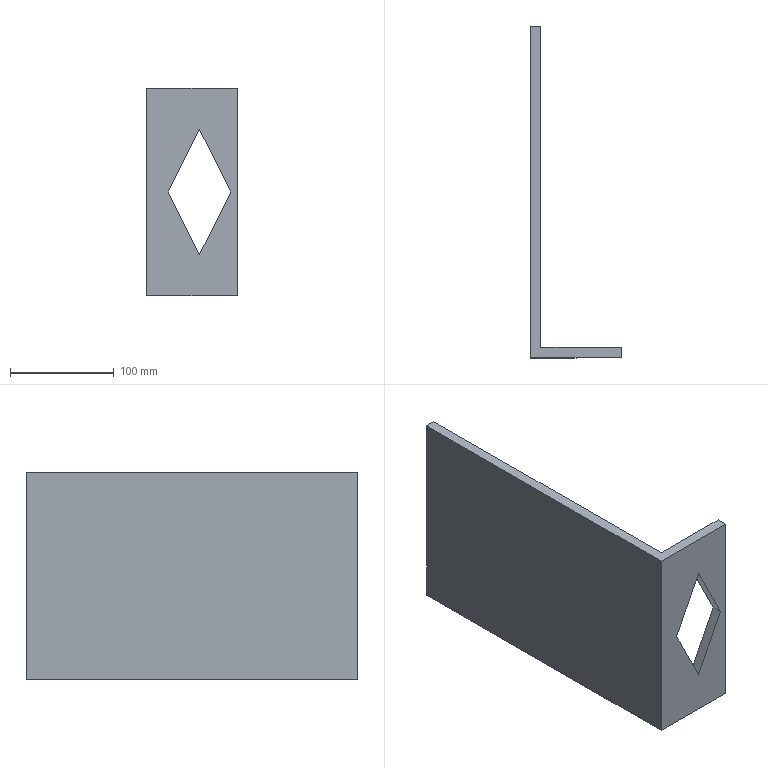Part | SolidWorks | features Cut 1, ExtruThin 1 | 1 solid | 12 faces | box 87.761 x 320 x 200 mm | volume 759523 mm3 | plane 12
STEP:
#1=CARTESIAN_POINT('',(-109.912,-100.,-180.));
#2=VERTEX_POINT('',#1);
#3=CARTESIAN_POINT('',(-139.912,-100.,-120.));
#4=VERTEX_POINT('',#3);
#5=CARTESIAN_POINT('',(-139.912,-100.,-120.));
#6=DIRECTION('',(-0.4472,0.,0.8944));
#7=VECTOR('',#6,1000.);
#8=LINE('',#5,#7);
#9=EDGE_CURVE('',#2,#4,#8,.T.);
#10=ORIENTED_EDGE('',*,*,#9,.F.);
#11=CARTESIAN_POINT('',(-139.912,-100.,-240.));
#12=VERTEX_POINT('',#11);
#13=CARTESIAN_POINT('',(-109.912,-100.,-180.));
#14=DIRECTION('',(0.4472,0.,0.8944));
#15=VECTOR('',#14,1000.);
#16=LINE('',#13,#15);
#17=EDGE_CURVE('',#12,#2,#16,.T.);
#18=ORIENTED_EDGE('',*,*,#17,.F.);
#19=CARTESIAN_POINT('',(-169.912,-100.,-180.));
#20=VERTEX_POINT('',#19);
#21=CARTESIAN_POINT('',(-139.912,-100.,-240.));
#22=DIRECTION('',(0.4472,0.,-0.8944));
#23=VECTOR('',#22,1000.);
#24=LINE('',#21,#23);
#25=EDGE_CURVE('',#20,#12,#24,.T.);
#26=ORIENTED_EDGE('',*,*,#25,.F.);
#27=CARTESIAN_POINT('',(-169.912,-100.,-180.));
#28=DIRECTION('',(-0.4472,0.,-0.8944));
#29=VECTOR('',#28,1000.);
#30=LINE('',#27,#29);
#31=EDGE_CURVE('',#4,#20,#30,.T.);
#32=ORIENTED_EDGE('',*,*,#31,.F.);
#33=EDGE_LOOP('',(#10,#18,#26,#32));
#34=FACE_BOUND('',#33,.T.);
#35=CARTESIAN_POINT('',(-191.016,-100.,-280.));
#36=VERTEX_POINT('',#35);
#37=CARTESIAN_POINT('',(-103.254,-100.,-280.));
#38=VERTEX_POINT('',#37);
#39=CARTESIAN_POINT('',(-191.016,-100.,-280.));
#40=DIRECTION('',(1.,0.,0.));
#41=VECTOR('',#40,1000.);
#42=LINE('',#39,#41);
#43=EDGE_CURVE('',#36,#38,#42,.T.);
#44=ORIENTED_EDGE('',*,*,#43,.T.);
#45=CARTESIAN_POINT('',(-103.254,-100.,-80.));
#46=VERTEX_POINT('',#45);
#47=CARTESIAN_POINT('',(-103.254,-100.,-80.));
#48=DIRECTION('',(0.,0.,-1.));
#49=VECTOR('',#48,1000.);
#50=LINE('',#47,#49);
#51=EDGE_CURVE('',#46,#38,#50,.T.);
#52=ORIENTED_EDGE('',*,*,#51,.F.);
#53=CARTESIAN_POINT('',(-191.016,-100.,-80.));
#54=VERTEX_POINT('',#53);
#55=CARTESIAN_POINT('',(-191.016,-100.,-80.));
#56=DIRECTION('',(1.,0.,0.));
#57=VECTOR('',#56,1000.);
#58=LINE('',#55,#57);
#59=EDGE_CURVE('',#54,#46,#58,.T.);
#60=ORIENTED_EDGE('',*,*,#59,.F.);
#61=CARTESIAN_POINT('',(-191.016,-100.,-80.));
#62=DIRECTION('',(0.,0.,-1.));
#63=VECTOR('',#62,1000.);
#64=LINE('',#61,#63);
#65=EDGE_CURVE('',#54,#36,#64,.T.);
#66=ORIENTED_EDGE('',*,*,#65,.T.);
#67=EDGE_LOOP('',(#44,#52,#60,#66));
#68=FACE_OUTER_BOUND('',#67,.T.);
#69=CARTESIAN_POINT('',(-191.016,-100.,-80.));
#70=DIRECTION('',(0.,1.,0.));
#71=DIRECTION('',(-1.,0.,0.));
#72=AXIS2_PLACEMENT_3D('',#69,#70,#71);
#73=PLANE('',#72);
#74=ADVANCED_FACE('',(#34,#68),#73,.F.);
#75=CARTESIAN_POINT('',(-103.254,-90.,-280.));
#76=VERTEX_POINT('',#75);
#77=CARTESIAN_POINT('',(-103.254,-90.,-280.));
#78=DIRECTION('',(0.,-1.,0.));
#79=VECTOR('',#78,1000.);
#80=LINE('',#77,#79);
#81=EDGE_CURVE('',#76,#38,#80,.T.);
#82=ORIENTED_EDGE('',*,*,#81,.F.);
#83=CARTESIAN_POINT('',(-103.254,-90.,-80.));
#84=VERTEX_POINT('',#83);
#85=CARTESIAN_POINT('',(-103.254,-90.,-80.));
#86=DIRECTION('',(0.,0.,-1.));
#87=VECTOR('',#86,1000.);
#88=LINE('',#85,#87);
#89=EDGE_CURVE('',#84,#76,#88,.T.);
#90=ORIENTED_EDGE('',*,*,#89,.F.);
#91=CARTESIAN_POINT('',(-103.254,-90.,-80.));
#92=DIRECTION('',(0.,-1.,0.));
#93=VECTOR('',#92,1000.);
#94=LINE('',#91,#93);
#95=EDGE_CURVE('',#84,#46,#94,.T.);
#96=ORIENTED_EDGE('',*,*,#95,.T.);
#97=ORIENTED_EDGE('',*,*,#51,.T.);
#98=EDGE_LOOP('',(#82,#90,#96,#97));
#99=FACE_OUTER_BOUND('',#98,.T.);
#100=CARTESIAN_POINT('',(-103.254,-90.,-80.));
#101=DIRECTION('',(1.,0.,0.));
#102=DIRECTION('',(0.,0.,-1.));
#103=AXIS2_PLACEMENT_3D('',#100,#101,#102);
#104=PLANE('',#103);
#105=ADVANCED_FACE('',(#99),#104,.T.);
#106=CARTESIAN_POINT('',(-109.912,-90.,-180.));
#107=VERTEX_POINT('',#106);
#108=CARTESIAN_POINT('',(-139.912,-90.,-240.));
#109=VERTEX_POINT('',#108);
#110=CARTESIAN_POINT('',(-86.132,-90.,-132.442));
#111=DIRECTION('',(-0.4472,0.,-0.8944));
#112=VECTOR('',#111,1000.);
#113=LINE('',#110,#112);
#114=EDGE_CURVE('',#107,#109,#113,.T.);
#115=ORIENTED_EDGE('',*,*,#114,.F.);
#116=CARTESIAN_POINT('',(-139.912,-90.,-120.));
#117=VERTEX_POINT('',#116);
#118=CARTESIAN_POINT('',(-166.132,-90.,-67.558));
#119=DIRECTION('',(0.4472,0.,-0.8944));
#120=VECTOR('',#119,1000.);
#121=LINE('',#118,#120);
#122=EDGE_CURVE('',#117,#107,#121,.T.);
#123=ORIENTED_EDGE('',*,*,#122,.F.);
#124=CARTESIAN_POINT('',(-169.912,-90.,-180.));
#125=VERTEX_POINT('',#124);
#126=CARTESIAN_POINT('',(-134.132,-90.,-108.442));
#127=DIRECTION('',(0.4472,0.,0.8944));
#128=VECTOR('',#127,1000.);
#129=LINE('',#126,#128);
#130=EDGE_CURVE('',#125,#117,#129,.T.);
#131=ORIENTED_EDGE('',*,*,#130,.F.);
#132=CARTESIAN_POINT('',(-214.132,-90.,-91.558));
#133=DIRECTION('',(-0.4472,0.,0.8944));
#134=VECTOR('',#133,1000.);
#135=LINE('',#132,#134);
#136=EDGE_CURVE('',#109,#125,#135,.T.);
#137=ORIENTED_EDGE('',*,*,#136,.F.);
#138=EDGE_LOOP('',(#115,#123,#131,#137));
#139=FACE_BOUND('',#138,.T.);
#140=CARTESIAN_POINT('',(-181.016,-90.,-280.));
#141=VERTEX_POINT('',#140);
#142=CARTESIAN_POINT('',(-191.016,-90.,-280.));
#143=DIRECTION('',(1.,0.,0.));
#144=VECTOR('',#143,1000.);
#145=LINE('',#142,#144);
#146=EDGE_CURVE('',#141,#76,#145,.T.);
#147=ORIENTED_EDGE('',*,*,#146,.F.);
#148=CARTESIAN_POINT('',(-181.016,-90.,-80.));
#149=VERTEX_POINT('',#148);
#150=CARTESIAN_POINT('',(-181.016,-90.,-80.));
#151=DIRECTION('',(0.,0.,-1.));
#152=VECTOR('',#151,1000.);
#153=LINE('',#150,#152);
#154=EDGE_CURVE('',#149,#141,#153,.T.);
#155=ORIENTED_EDGE('',*,*,#154,.F.);
#156=CARTESIAN_POINT('',(-191.016,-90.,-80.));
#157=DIRECTION('',(1.,0.,0.));
#158=VECTOR('',#157,1000.);
#159=LINE('',#156,#158);
#160=EDGE_CURVE('',#149,#84,#159,.T.);
#161=ORIENTED_EDGE('',*,*,#160,.T.);
#162=ORIENTED_EDGE('',*,*,#89,.T.);
#163=EDGE_LOOP('',(#147,#155,#161,#162));
#164=FACE_OUTER_BOUND('',#163,.T.);
#165=CARTESIAN_POINT('',(-191.016,-90.,-80.));
#166=DIRECTION('',(0.,1.,0.));
#167=DIRECTION('',(-1.,0.,0.));
#168=AXIS2_PLACEMENT_3D('',#165,#166,#167);
#169=PLANE('',#168);
#170=ADVANCED_FACE('',(#139,#164),#169,.T.);
#171=CARTESIAN_POINT('',(-181.016,220.,-280.));
#172=VERTEX_POINT('',#171);
#173=CARTESIAN_POINT('',(-181.016,220.,-280.));
#174=DIRECTION('',(0.,-1.,0.));
#175=VECTOR('',#174,1000.);
#176=LINE('',#173,#175);
#177=EDGE_CURVE('',#172,#141,#176,.T.);
#178=ORIENTED_EDGE('',*,*,#177,.F.);
#179=CARTESIAN_POINT('',(-181.016,220.,-80.));
#180=VERTEX_POINT('',#179);
#181=CARTESIAN_POINT('',(-181.016,220.,-80.));
#182=DIRECTION('',(0.,0.,-1.));
#183=VECTOR('',#182,1000.);
#184=LINE('',#181,#183);
#185=EDGE_CURVE('',#180,#172,#184,.T.);
#186=ORIENTED_EDGE('',*,*,#185,.F.);
#187=CARTESIAN_POINT('',(-181.016,220.,-80.));
#188=DIRECTION('',(0.,-1.,0.));
#189=VECTOR('',#188,1000.);
#190=LINE('',#187,#189);
#191=EDGE_CURVE('',#180,#149,#190,.T.);
#192=ORIENTED_EDGE('',*,*,#191,.T.);
#193=ORIENTED_EDGE('',*,*,#154,.T.);
#194=EDGE_LOOP('',(#178,#186,#192,#193));
#195=FACE_OUTER_BOUND('',#194,.T.);
#196=CARTESIAN_POINT('',(-181.016,220.,-80.));
#197=DIRECTION('',(1.,0.,0.));
#198=DIRECTION('',(0.,1.,0.));
#199=AXIS2_PLACEMENT_3D('',#196,#197,#198);
#200=PLANE('',#199);
#201=ADVANCED_FACE('',(#195),#200,.T.);
#202=CARTESIAN_POINT('',(-191.016,220.,-280.));
#203=VERTEX_POINT('',#202);
#204=CARTESIAN_POINT('',(-191.016,220.,-280.));
#205=DIRECTION('',(1.,0.,0.));
#206=VECTOR('',#205,1000.);
#207=LINE('',#204,#206);
#208=EDGE_CURVE('',#203,#172,#207,.T.);
#209=ORIENTED_EDGE('',*,*,#208,.F.);
#210=CARTESIAN_POINT('',(-191.016,220.,-80.));
#211=VERTEX_POINT('',#210);
#212=CARTESIAN_POINT('',(-191.016,220.,-80.));
#213=DIRECTION('',(0.,0.,-1.));
#214=VECTOR('',#213,1000.);
#215=LINE('',#212,#214);
#216=EDGE_CURVE('',#211,#203,#215,.T.);
#217=ORIENTED_EDGE('',*,*,#216,.F.);
#218=CARTESIAN_POINT('',(-191.016,220.,-80.));
#219=DIRECTION('',(1.,0.,0.));
#220=VECTOR('',#219,1000.);
#221=LINE('',#218,#220);
#222=EDGE_CURVE('',#211,#180,#221,.T.);
#223=ORIENTED_EDGE('',*,*,#222,.T.);
#224=ORIENTED_EDGE('',*,*,#185,.T.);
#225=EDGE_LOOP('',(#209,#217,#223,#224));
#226=FACE_OUTER_BOUND('',#225,.T.);
#227=CARTESIAN_POINT('',(-191.016,220.,-80.));
#228=DIRECTION('',(0.,1.,0.));
#229=DIRECTION('',(0.,0.,1.));
#230=AXIS2_PLACEMENT_3D('',#227,#228,#229);
#231=PLANE('',#230);
#232=ADVANCED_FACE('',(#226),#231,.T.);
#233=CARTESIAN_POINT('',(-191.016,220.,-280.));
#234=DIRECTION('',(0.,-1.,0.));
#235=VECTOR('',#234,1000.);
#236=LINE('',#233,#235);
#237=EDGE_CURVE('',#203,#36,#236,.T.);
#238=ORIENTED_EDGE('',*,*,#237,.T.);
#239=ORIENTED_EDGE('',*,*,#65,.F.);
#240=CARTESIAN_POINT('',(-191.016,220.,-80.));
#241=DIRECTION('',(0.,-1.,0.));
#242=VECTOR('',#241,1000.);
#243=LINE('',#240,#242);
#244=EDGE_CURVE('',#211,#54,#243,.T.);
#245=ORIENTED_EDGE('',*,*,#244,.F.);
#246=ORIENTED_EDGE('',*,*,#216,.T.);
#247=EDGE_LOOP('',(#238,#239,#245,#246));
#248=FACE_OUTER_BOUND('',#247,.T.);
#249=CARTESIAN_POINT('',(-191.016,220.,-80.));
#250=DIRECTION('',(1.,0.,0.));
#251=DIRECTION('',(0.,1.,0.));
#252=AXIS2_PLACEMENT_3D('',#249,#250,#251);
#253=PLANE('',#252);
#254=ADVANCED_FACE('',(#248),#253,.F.);
#255=ORIENTED_EDGE('',*,*,#59,.T.);
#256=ORIENTED_EDGE('',*,*,#95,.F.);
#257=ORIENTED_EDGE('',*,*,#160,.F.);
#258=ORIENTED_EDGE('',*,*,#191,.F.);
#259=ORIENTED_EDGE('',*,*,#222,.F.);
#260=ORIENTED_EDGE('',*,*,#244,.T.);
#261=EDGE_LOOP('',(#255,#256,#257,#258,#259,#260));
#262=FACE_OUTER_BOUND('',#261,.T.);
#263=CARTESIAN_POINT('',(0.,0.,-80.));
#264=DIRECTION('',(0.,0.,-1.));
#265=DIRECTION('',(-1.,0.,0.));
#266=AXIS2_PLACEMENT_3D('',#263,#264,#265);
#267=PLANE('',#266);
#268=ADVANCED_FACE('',(#262),#267,.F.);
#269=ORIENTED_EDGE('',*,*,#43,.F.);
#270=ORIENTED_EDGE('',*,*,#237,.F.);
#271=ORIENTED_EDGE('',*,*,#208,.T.);
#272=ORIENTED_EDGE('',*,*,#177,.T.);
#273=ORIENTED_EDGE('',*,*,#146,.T.);
#274=ORIENTED_EDGE('',*,*,#81,.T.);
#275=EDGE_LOOP('',(#269,#270,#271,#272,#273,#274));
#276=FACE_OUTER_BOUND('',#275,.T.);
#277=CARTESIAN_POINT('',(0.,0.,-280.));
#278=DIRECTION('',(0.,0.,-1.));
#279=DIRECTION('',(-1.,0.,0.));
#280=AXIS2_PLACEMENT_3D('',#277,#278,#279);
#281=PLANE('',#280);
#282=ADVANCED_FACE('',(#276),#281,.T.);
#283=ORIENTED_EDGE('',*,*,#114,.T.);
#284=CARTESIAN_POINT('',(-139.912,-21.,-240.));
#285=DIRECTION('',(0.,-1.,0.));
#286=VECTOR('',#285,1000.);
#287=LINE('',#284,#286);
#288=EDGE_CURVE('',#109,#12,#287,.T.);
#289=ORIENTED_EDGE('',*,*,#288,.T.);
#290=ORIENTED_EDGE('',*,*,#17,.T.);
#291=CARTESIAN_POINT('',(-109.912,-21.,-180.));
#292=DIRECTION('',(0.,-1.,0.));
#293=VECTOR('',#292,1000.);
#294=LINE('',#291,#293);
#295=EDGE_CURVE('',#107,#2,#294,.T.);
#296=ORIENTED_EDGE('',*,*,#295,.F.);
#297=EDGE_LOOP('',(#283,#289,#290,#296));
#298=FACE_OUTER_BOUND('',#297,.T.);
#299=CARTESIAN_POINT('',(-109.912,-21.,-180.));
#300=DIRECTION('',(0.8944,0.,-0.4472));
#301=DIRECTION('',(-0.4472,0.,-0.8944));
#302=AXIS2_PLACEMENT_3D('',#299,#300,#301);
#303=PLANE('',#302);
#304=ADVANCED_FACE('',(#298),#303,.F.);
#305=ORIENTED_EDGE('',*,*,#136,.T.);
#306=CARTESIAN_POINT('',(-169.912,-21.,-180.));
#307=DIRECTION('',(0.,-1.,0.));
#308=VECTOR('',#307,1000.);
#309=LINE('',#306,#308);
#310=EDGE_CURVE('',#125,#20,#309,.T.);
#311=ORIENTED_EDGE('',*,*,#310,.T.);
#312=ORIENTED_EDGE('',*,*,#25,.T.);
#313=ORIENTED_EDGE('',*,*,#288,.F.);
#314=EDGE_LOOP('',(#305,#311,#312,#313));
#315=FACE_OUTER_BOUND('',#314,.T.);
#316=CARTESIAN_POINT('',(-139.912,-21.,-240.));
#317=DIRECTION('',(-0.8944,0.,-0.4472));
#318=DIRECTION('',(-0.4472,0.,0.8944));
#319=AXIS2_PLACEMENT_3D('',#316,#317,#318);
#320=PLANE('',#319);
#321=ADVANCED_FACE('',(#315),#320,.F.);
#322=ORIENTED_EDGE('',*,*,#130,.T.);
#323=CARTESIAN_POINT('',(-139.912,-21.,-120.));
#324=DIRECTION('',(0.,-1.,0.));
#325=VECTOR('',#324,1000.);
#326=LINE('',#323,#325);
#327=EDGE_CURVE('',#117,#4,#326,.T.);
#328=ORIENTED_EDGE('',*,*,#327,.T.);
#329=ORIENTED_EDGE('',*,*,#31,.T.);
#330=ORIENTED_EDGE('',*,*,#310,.F.);
#331=EDGE_LOOP('',(#322,#328,#329,#330));
#332=FACE_OUTER_BOUND('',#331,.T.);
#333=CARTESIAN_POINT('',(-169.912,-21.,-180.));
#334=DIRECTION('',(-0.8944,0.,0.4472));
#335=DIRECTION('',(0.4472,0.,0.8944));
#336=AXIS2_PLACEMENT_3D('',#333,#334,#335);
#337=PLANE('',#336);
#338=ADVANCED_FACE('',(#332),#337,.F.);
#339=ORIENTED_EDGE('',*,*,#122,.T.);
#340=ORIENTED_EDGE('',*,*,#295,.T.);
#341=ORIENTED_EDGE('',*,*,#9,.T.);
#342=ORIENTED_EDGE('',*,*,#327,.F.);
#343=EDGE_LOOP('',(#339,#340,#341,#342));
#344=FACE_OUTER_BOUND('',#343,.T.);
#345=CARTESIAN_POINT('',(-139.912,-21.,-120.));
#346=DIRECTION('',(0.8944,0.,0.4472));
#347=DIRECTION('',(0.4472,0.,-0.8944));
#348=AXIS2_PLACEMENT_3D('',#345,#346,#347);
#349=PLANE('',#348);
#350=ADVANCED_FACE('',(#344),#349,.F.);
#351=CLOSED_SHELL('',(#74,#105,#170,#201,#232,#254,#268,#282,#304,#321,#338,#350));
#352=MANIFOLD_SOLID_BREP('',#351);
#353=CARTESIAN_POINT('',(0.,0.,0.));
#354=DIRECTION('',(0.,0.,1.));
#355=DIRECTION('',(1.,0.,0.));
#356=AXIS2_PLACEMENT_3D('',#353,#354,#355);
#357=(LENGTH_UNIT()NAMED_UNIT(*)SI_UNIT(.MILLI.,.METRE.));
#358=UNCERTAINTY_MEASURE_WITH_UNIT(LENGTH_MEASURE(0.00001),#357,'','');
#359=(NAMED_UNIT(*)PLANE_ANGLE_UNIT()SI_UNIT($,.RADIAN.));
#360=(NAMED_UNIT(*)SI_UNIT($,.STERADIAN.)SOLID_ANGLE_UNIT());
#361=(GEOMETRIC_REPRESENTATION_CONTEXT(3)GLOBAL_UNCERTAINTY_ASSIGNED_CONTEXT((#358))GLOBAL_UNIT_ASSIGNED_CONTEXT((#357,#359,#360))REPRESENTATION_CONTEXT('',''));
#362=ADVANCED_BREP_SHAPE_REPRESENTATION('',(#352,#356),#361);